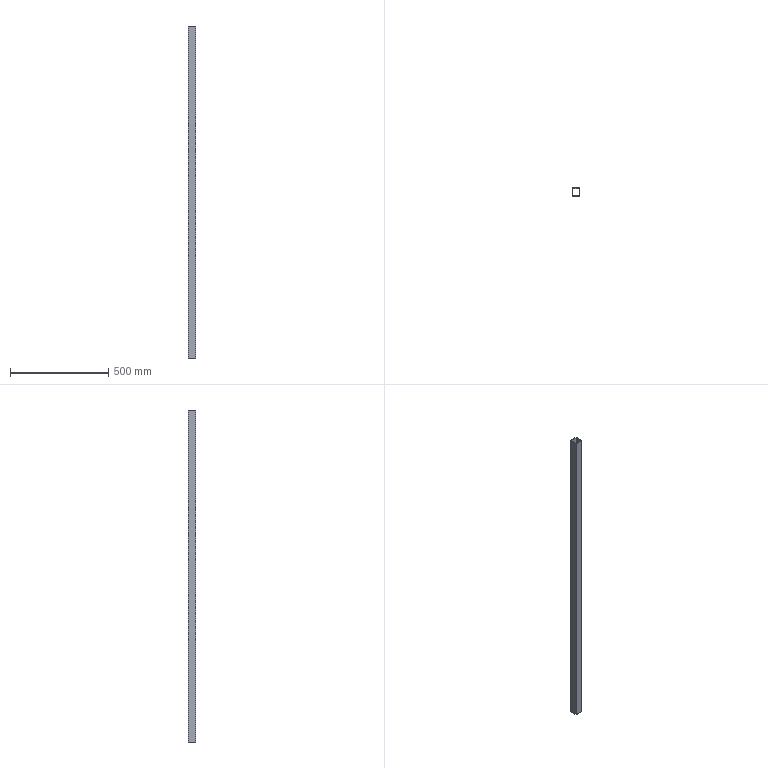Part | STEP file | BCC3 H18_6 | 1 solid | 10 faces | box 40 x 40 x 1690 mm | volume 750360 mm3 | plane 10
STEP:
#1=CARTESIAN_POINT('',(0.,0.,0.));
#2=DIRECTION('',(0.,0.,1.));
#3=DIRECTION('',(1.,0.,0.));
#4=AXIS2_PLACEMENT_3D('',#1,#2,#3);
#5=CARTESIAN_POINT('',(-20.,20.,845.));
#6=VERTEX_POINT('',#5);
#7=CARTESIAN_POINT('',(-20.,-20.,845.));
#8=VERTEX_POINT('',#7);
#9=CARTESIAN_POINT('',(-20.,20.,845.));
#10=DIRECTION('',(0.,-1.,0.));
#11=VECTOR('',#10,1.);
#12=LINE('',#9,#11);
#13=CARTESIAN_POINT('',(0.,0.,845.));
#14=DIRECTION('',(0.,0.,1.));
#15=DIRECTION('',(1.,0.,0.));
#16=AXIS2_PLACEMENT_3D('',#13,#14,#15);
#17=PLANE('',#16);
#18=CARTESIAN_POINT('',(-20.,20.));
#19=DIRECTION('',(0.,-1.));
#20=VECTOR('',#19,1.);
#21=LINE('',#18,#20);
#22=(GEOMETRIC_REPRESENTATION_CONTEXT(2)PARAMETRIC_REPRESENTATION_CONTEXT()REPRESENTATION_CONTEXT('',''));
#23=DEFINITIONAL_REPRESENTATION('',(#21),#22);
#24=PCURVE('',#17,#23);
#25=CARTESIAN_POINT('',(-20.,20.,845.));
#26=DIRECTION('',(1.,0.,0.));
#27=DIRECTION('',(0.,1.,0.));
#28=AXIS2_PLACEMENT_3D('',#25,#26,#27);
#29=PLANE('',#28);
#30=CARTESIAN_POINT('',(0.,0.));
#31=DIRECTION('',(-1.,0.));
#32=VECTOR('',#31,1.);
#33=LINE('',#30,#32);
#34=(GEOMETRIC_REPRESENTATION_CONTEXT(2)PARAMETRIC_REPRESENTATION_CONTEXT()REPRESENTATION_CONTEXT('',''));
#35=DEFINITIONAL_REPRESENTATION('',(#33),#34);
#36=PCURVE('',#29,#35);
#37=SURFACE_CURVE('',#12,(#24,#36),.PCURVE_S1.);
#38=EDGE_CURVE('',#6,#8,#37,.T.);
#39=ORIENTED_EDGE('',*,*,#38,.T.);
#40=CARTESIAN_POINT('',(20.,-20.,845.));
#41=VERTEX_POINT('',#40);
#42=CARTESIAN_POINT('',(-20.,-20.,845.));
#43=DIRECTION('',(1.,0.,0.));
#44=VECTOR('',#43,1.);
#45=LINE('',#42,#44);
#46=CARTESIAN_POINT('',(-20.,-20.));
#47=DIRECTION('',(1.,0.));
#48=VECTOR('',#47,1.);
#49=LINE('',#46,#48);
#50=(GEOMETRIC_REPRESENTATION_CONTEXT(2)PARAMETRIC_REPRESENTATION_CONTEXT()REPRESENTATION_CONTEXT('',''));
#51=DEFINITIONAL_REPRESENTATION('',(#49),#50);
#52=PCURVE('',#17,#51);
#53=CARTESIAN_POINT('',(-20.,-20.,845.));
#54=DIRECTION('',(0.,1.,0.));
#55=DIRECTION('',(0.,0.,1.));
#56=AXIS2_PLACEMENT_3D('',#53,#54,#55);
#57=PLANE('',#56);
#58=CARTESIAN_POINT('',(0.,0.));
#59=DIRECTION('',(0.,1.));
#60=VECTOR('',#59,1.);
#61=LINE('',#58,#60);
#62=(GEOMETRIC_REPRESENTATION_CONTEXT(2)PARAMETRIC_REPRESENTATION_CONTEXT()REPRESENTATION_CONTEXT('',''));
#63=DEFINITIONAL_REPRESENTATION('',(#61),#62);
#64=PCURVE('',#57,#63);
#65=SURFACE_CURVE('',#45,(#52,#64),.PCURVE_S1.);
#66=EDGE_CURVE('',#8,#41,#65,.T.);
#67=ORIENTED_EDGE('',*,*,#66,.T.);
#68=CARTESIAN_POINT('',(20.,20.,845.));
#69=VERTEX_POINT('',#68);
#70=CARTESIAN_POINT('',(20.,20.,845.));
#71=DIRECTION('',(0.,1.,0.));
#72=VECTOR('',#71,1.);
#73=LINE('',#70,#72);
#74=CARTESIAN_POINT('',(20.,20.));
#75=DIRECTION('',(0.,1.));
#76=VECTOR('',#75,1.);
#77=LINE('',#74,#76);
#78=(GEOMETRIC_REPRESENTATION_CONTEXT(2)PARAMETRIC_REPRESENTATION_CONTEXT()REPRESENTATION_CONTEXT('',''));
#79=DEFINITIONAL_REPRESENTATION('',(#77),#78);
#80=PCURVE('',#17,#79);
#81=CARTESIAN_POINT('',(20.,20.,845.));
#82=DIRECTION('',(-1.,0.,0.));
#83=DIRECTION('',(0.,-1.,0.));
#84=AXIS2_PLACEMENT_3D('',#81,#82,#83);
#85=PLANE('',#84);
#86=CARTESIAN_POINT('',(0.,0.));
#87=DIRECTION('',(-1.,0.));
#88=VECTOR('',#87,1.);
#89=LINE('',#86,#88);
#90=(GEOMETRIC_REPRESENTATION_CONTEXT(2)PARAMETRIC_REPRESENTATION_CONTEXT()REPRESENTATION_CONTEXT('',''));
#91=DEFINITIONAL_REPRESENTATION('',(#89),#90);
#92=PCURVE('',#85,#91);
#93=SURFACE_CURVE('',#73,(#80,#92),.PCURVE_S1.);
#94=EDGE_CURVE('',#41,#69,#93,.T.);
#95=ORIENTED_EDGE('',*,*,#94,.T.);
#96=CARTESIAN_POINT('',(-20.,20.,845.));
#97=DIRECTION('',(-1.,0.,0.));
#98=VECTOR('',#97,1.);
#99=LINE('',#96,#98);
#100=CARTESIAN_POINT('',(-20.,20.));
#101=DIRECTION('',(-1.,0.));
#102=VECTOR('',#101,1.);
#103=LINE('',#100,#102);
#104=(GEOMETRIC_REPRESENTATION_CONTEXT(2)PARAMETRIC_REPRESENTATION_CONTEXT()REPRESENTATION_CONTEXT('',''));
#105=DEFINITIONAL_REPRESENTATION('',(#103),#104);
#106=PCURVE('',#17,#105);
#107=CARTESIAN_POINT('',(-20.,20.,845.));
#108=DIRECTION('',(0.,-1.,0.));
#109=DIRECTION('',(0.,0.,-1.));
#110=AXIS2_PLACEMENT_3D('',#107,#108,#109);
#111=PLANE('',#110);
#112=CARTESIAN_POINT('',(0.,0.));
#113=DIRECTION('',(0.,-1.));
#114=VECTOR('',#113,1.);
#115=LINE('',#112,#114);
#116=(GEOMETRIC_REPRESENTATION_CONTEXT(2)PARAMETRIC_REPRESENTATION_CONTEXT()REPRESENTATION_CONTEXT('',''));
#117=DEFINITIONAL_REPRESENTATION('',(#115),#116);
#118=PCURVE('',#111,#117);
#119=SURFACE_CURVE('',#99,(#106,#118),.PCURVE_S1.);
#120=EDGE_CURVE('',#69,#6,#119,.T.);
#121=ORIENTED_EDGE('',*,*,#120,.T.);
#122=EDGE_LOOP('',(#39,#67,#95,#121));
#123=FACE_BOUND('',#122,.T.);
#124=CARTESIAN_POINT('',(-17.,-17.,845.));
#125=VERTEX_POINT('',#124);
#126=CARTESIAN_POINT('',(17.,-17.,845.));
#127=VERTEX_POINT('',#126);
#128=CARTESIAN_POINT('',(-17.,-17.,845.));
#129=DIRECTION('',(1.,0.,0.));
#130=VECTOR('',#129,1.);
#131=LINE('',#128,#130);
#132=CARTESIAN_POINT('',(-17.,-17.));
#133=DIRECTION('',(1.,0.));
#134=VECTOR('',#133,1.);
#135=LINE('',#132,#134);
#136=(GEOMETRIC_REPRESENTATION_CONTEXT(2)PARAMETRIC_REPRESENTATION_CONTEXT()REPRESENTATION_CONTEXT('',''));
#137=DEFINITIONAL_REPRESENTATION('',(#135),#136);
#138=PCURVE('',#17,#137);
#139=CARTESIAN_POINT('',(-17.,-17.,845.));
#140=DIRECTION('',(0.,1.,0.));
#141=DIRECTION('',(-1.,0.,0.));
#142=AXIS2_PLACEMENT_3D('',#139,#140,#141);
#143=PLANE('',#142);
#144=CARTESIAN_POINT('',(0.,0.));
#145=DIRECTION('',(-1.,0.));
#146=VECTOR('',#145,1.);
#147=LINE('',#144,#146);
#148=(GEOMETRIC_REPRESENTATION_CONTEXT(2)PARAMETRIC_REPRESENTATION_CONTEXT()REPRESENTATION_CONTEXT('',''));
#149=DEFINITIONAL_REPRESENTATION('',(#147),#148);
#150=PCURVE('',#143,#149);
#151=SURFACE_CURVE('',#131,(#138,#150),.PCURVE_S1.);
#152=EDGE_CURVE('',#125,#127,#151,.T.);
#153=ORIENTED_EDGE('',*,*,#152,.F.);
#154=CARTESIAN_POINT('',(-17.,17.,845.));
#155=VERTEX_POINT('',#154);
#156=CARTESIAN_POINT('',(-17.,17.,845.));
#157=DIRECTION('',(0.,-1.,0.));
#158=VECTOR('',#157,1.);
#159=LINE('',#156,#158);
#160=CARTESIAN_POINT('',(-17.,17.));
#161=DIRECTION('',(0.,-1.));
#162=VECTOR('',#161,1.);
#163=LINE('',#160,#162);
#164=(GEOMETRIC_REPRESENTATION_CONTEXT(2)PARAMETRIC_REPRESENTATION_CONTEXT()REPRESENTATION_CONTEXT('',''));
#165=DEFINITIONAL_REPRESENTATION('',(#163),#164);
#166=PCURVE('',#17,#165);
#167=CARTESIAN_POINT('',(-17.,17.,845.));
#168=DIRECTION('',(1.,0.,0.));
#169=DIRECTION('',(0.,1.,0.));
#170=AXIS2_PLACEMENT_3D('',#167,#168,#169);
#171=PLANE('',#170);
#172=CARTESIAN_POINT('',(0.,0.));
#173=DIRECTION('',(-1.,0.));
#174=VECTOR('',#173,1.);
#175=LINE('',#172,#174);
#176=(GEOMETRIC_REPRESENTATION_CONTEXT(2)PARAMETRIC_REPRESENTATION_CONTEXT()REPRESENTATION_CONTEXT('',''));
#177=DEFINITIONAL_REPRESENTATION('',(#175),#176);
#178=PCURVE('',#171,#177);
#179=SURFACE_CURVE('',#159,(#166,#178),.PCURVE_S1.);
#180=EDGE_CURVE('',#155,#125,#179,.T.);
#181=ORIENTED_EDGE('',*,*,#180,.F.);
#182=CARTESIAN_POINT('',(17.,17.,845.));
#183=VERTEX_POINT('',#182);
#184=CARTESIAN_POINT('',(-17.,17.,845.));
#185=DIRECTION('',(-1.,0.,0.));
#186=VECTOR('',#185,1.);
#187=LINE('',#184,#186);
#188=CARTESIAN_POINT('',(-17.,17.));
#189=DIRECTION('',(-1.,0.));
#190=VECTOR('',#189,1.);
#191=LINE('',#188,#190);
#192=(GEOMETRIC_REPRESENTATION_CONTEXT(2)PARAMETRIC_REPRESENTATION_CONTEXT()REPRESENTATION_CONTEXT('',''));
#193=DEFINITIONAL_REPRESENTATION('',(#191),#192);
#194=PCURVE('',#17,#193);
#195=CARTESIAN_POINT('',(-17.,17.,845.));
#196=DIRECTION('',(0.,-1.,0.));
#197=DIRECTION('',(0.,0.,-1.));
#198=AXIS2_PLACEMENT_3D('',#195,#196,#197);
#199=PLANE('',#198);
#200=CARTESIAN_POINT('',(0.,0.));
#201=DIRECTION('',(0.,-1.));
#202=VECTOR('',#201,1.);
#203=LINE('',#200,#202);
#204=(GEOMETRIC_REPRESENTATION_CONTEXT(2)PARAMETRIC_REPRESENTATION_CONTEXT()REPRESENTATION_CONTEXT('',''));
#205=DEFINITIONAL_REPRESENTATION('',(#203),#204);
#206=PCURVE('',#199,#205);
#207=SURFACE_CURVE('',#187,(#194,#206),.PCURVE_S1.);
#208=EDGE_CURVE('',#183,#155,#207,.T.);
#209=ORIENTED_EDGE('',*,*,#208,.F.);
#210=CARTESIAN_POINT('',(17.,17.,845.));
#211=DIRECTION('',(0.,1.,0.));
#212=VECTOR('',#211,1.);
#213=LINE('',#210,#212);
#214=CARTESIAN_POINT('',(17.,17.));
#215=DIRECTION('',(0.,1.));
#216=VECTOR('',#215,1.);
#217=LINE('',#214,#216);
#218=(GEOMETRIC_REPRESENTATION_CONTEXT(2)PARAMETRIC_REPRESENTATION_CONTEXT()REPRESENTATION_CONTEXT('',''));
#219=DEFINITIONAL_REPRESENTATION('',(#217),#218);
#220=PCURVE('',#17,#219);
#221=CARTESIAN_POINT('',(17.,17.,845.));
#222=DIRECTION('',(-1.,0.,0.));
#223=DIRECTION('',(0.,-1.,0.));
#224=AXIS2_PLACEMENT_3D('',#221,#222,#223);
#225=PLANE('',#224);
#226=CARTESIAN_POINT('',(0.,0.));
#227=DIRECTION('',(-1.,0.));
#228=VECTOR('',#227,1.);
#229=LINE('',#226,#228);
#230=(GEOMETRIC_REPRESENTATION_CONTEXT(2)PARAMETRIC_REPRESENTATION_CONTEXT()REPRESENTATION_CONTEXT('',''));
#231=DEFINITIONAL_REPRESENTATION('',(#229),#230);
#232=PCURVE('',#225,#231);
#233=SURFACE_CURVE('',#213,(#220,#232),.PCURVE_S1.);
#234=EDGE_CURVE('',#127,#183,#233,.T.);
#235=ORIENTED_EDGE('',*,*,#234,.F.);
#236=EDGE_LOOP('',(#153,#181,#209,#235));
#237=FACE_BOUND('',#236,.T.);
#238=ADVANCED_FACE('',(#123,#237),#17,.T.);
#239=CARTESIAN_POINT('',(-20.,20.,-845.));
#240=VERTEX_POINT('',#239);
#241=CARTESIAN_POINT('',(-20.,-20.,-845.));
#242=VERTEX_POINT('',#241);
#243=CARTESIAN_POINT('',(-20.,20.,-845.));
#244=DIRECTION('',(0.,-1.,0.));
#245=VECTOR('',#244,1.);
#246=LINE('',#243,#245);
#247=CARTESIAN_POINT('',(0.,0.,-845.));
#248=DIRECTION('',(0.,0.,1.));
#249=DIRECTION('',(1.,0.,0.));
#250=AXIS2_PLACEMENT_3D('',#247,#248,#249);
#251=PLANE('',#250);
#252=CARTESIAN_POINT('',(-20.,20.));
#253=DIRECTION('',(0.,-1.));
#254=VECTOR('',#253,1.);
#255=LINE('',#252,#254);
#256=(GEOMETRIC_REPRESENTATION_CONTEXT(2)PARAMETRIC_REPRESENTATION_CONTEXT()REPRESENTATION_CONTEXT('',''));
#257=DEFINITIONAL_REPRESENTATION('',(#255),#256);
#258=PCURVE('',#251,#257);
#259=CARTESIAN_POINT('',(0.,-1690.));
#260=DIRECTION('',(-1.,0.));
#261=VECTOR('',#260,1.);
#262=LINE('',#259,#261);
#263=(GEOMETRIC_REPRESENTATION_CONTEXT(2)PARAMETRIC_REPRESENTATION_CONTEXT()REPRESENTATION_CONTEXT('',''));
#264=DEFINITIONAL_REPRESENTATION('',(#262),#263);
#265=PCURVE('',#29,#264);
#266=SURFACE_CURVE('',#246,(#258,#265),.PCURVE_S1.);
#267=EDGE_CURVE('',#240,#242,#266,.T.);
#268=ORIENTED_EDGE('',*,*,#267,.F.);
#269=CARTESIAN_POINT('',(20.,20.,-845.));
#270=VERTEX_POINT('',#269);
#271=CARTESIAN_POINT('',(-20.,20.,-845.));
#272=DIRECTION('',(-1.,0.,0.));
#273=VECTOR('',#272,1.);
#274=LINE('',#271,#273);
#275=CARTESIAN_POINT('',(-20.,20.));
#276=DIRECTION('',(-1.,0.));
#277=VECTOR('',#276,1.);
#278=LINE('',#275,#277);
#279=(GEOMETRIC_REPRESENTATION_CONTEXT(2)PARAMETRIC_REPRESENTATION_CONTEXT()REPRESENTATION_CONTEXT('',''));
#280=DEFINITIONAL_REPRESENTATION('',(#278),#279);
#281=PCURVE('',#251,#280);
#282=CARTESIAN_POINT('',(1690.,0.));
#283=DIRECTION('',(0.,-1.));
#284=VECTOR('',#283,1.);
#285=LINE('',#282,#284);
#286=(GEOMETRIC_REPRESENTATION_CONTEXT(2)PARAMETRIC_REPRESENTATION_CONTEXT()REPRESENTATION_CONTEXT('',''));
#287=DEFINITIONAL_REPRESENTATION('',(#285),#286);
#288=PCURVE('',#111,#287);
#289=SURFACE_CURVE('',#274,(#281,#288),.PCURVE_S1.);
#290=EDGE_CURVE('',#270,#240,#289,.T.);
#291=ORIENTED_EDGE('',*,*,#290,.F.);
#292=CARTESIAN_POINT('',(20.,-20.,-845.));
#293=VERTEX_POINT('',#292);
#294=CARTESIAN_POINT('',(20.,20.,-845.));
#295=DIRECTION('',(0.,1.,0.));
#296=VECTOR('',#295,1.);
#297=LINE('',#294,#296);
#298=CARTESIAN_POINT('',(20.,20.));
#299=DIRECTION('',(0.,1.));
#300=VECTOR('',#299,1.);
#301=LINE('',#298,#300);
#302=(GEOMETRIC_REPRESENTATION_CONTEXT(2)PARAMETRIC_REPRESENTATION_CONTEXT()REPRESENTATION_CONTEXT('',''));
#303=DEFINITIONAL_REPRESENTATION('',(#301),#302);
#304=PCURVE('',#251,#303);
#305=CARTESIAN_POINT('',(0.,-1690.));
#306=DIRECTION('',(-1.,0.));
#307=VECTOR('',#306,1.);
#308=LINE('',#305,#307);
#309=(GEOMETRIC_REPRESENTATION_CONTEXT(2)PARAMETRIC_REPRESENTATION_CONTEXT()REPRESENTATION_CONTEXT('',''));
#310=DEFINITIONAL_REPRESENTATION('',(#308),#309);
#311=PCURVE('',#85,#310);
#312=SURFACE_CURVE('',#297,(#304,#311),.PCURVE_S1.);
#313=EDGE_CURVE('',#293,#270,#312,.T.);
#314=ORIENTED_EDGE('',*,*,#313,.F.);
#315=CARTESIAN_POINT('',(-20.,-20.,-845.));
#316=DIRECTION('',(1.,0.,0.));
#317=VECTOR('',#316,1.);
#318=LINE('',#315,#317);
#319=CARTESIAN_POINT('',(-20.,-20.));
#320=DIRECTION('',(1.,0.));
#321=VECTOR('',#320,1.);
#322=LINE('',#319,#321);
#323=(GEOMETRIC_REPRESENTATION_CONTEXT(2)PARAMETRIC_REPRESENTATION_CONTEXT()REPRESENTATION_CONTEXT('',''));
#324=DEFINITIONAL_REPRESENTATION('',(#322),#323);
#325=PCURVE('',#251,#324);
#326=CARTESIAN_POINT('',(-1690.,0.));
#327=DIRECTION('',(0.,1.));
#328=VECTOR('',#327,1.);
#329=LINE('',#326,#328);
#330=(GEOMETRIC_REPRESENTATION_CONTEXT(2)PARAMETRIC_REPRESENTATION_CONTEXT()REPRESENTATION_CONTEXT('',''));
#331=DEFINITIONAL_REPRESENTATION('',(#329),#330);
#332=PCURVE('',#57,#331);
#333=SURFACE_CURVE('',#318,(#325,#332),.PCURVE_S1.);
#334=EDGE_CURVE('',#242,#293,#333,.T.);
#335=ORIENTED_EDGE('',*,*,#334,.F.);
#336=EDGE_LOOP('',(#268,#291,#314,#335));
#337=FACE_BOUND('',#336,.T.);
#338=CARTESIAN_POINT('',(-17.,17.,-845.));
#339=VERTEX_POINT('',#338);
#340=CARTESIAN_POINT('',(-17.,-17.,-845.));
#341=VERTEX_POINT('',#340);
#342=CARTESIAN_POINT('',(-17.,17.,-845.));
#343=DIRECTION('',(0.,-1.,0.));
#344=VECTOR('',#343,1.);
#345=LINE('',#342,#344);
#346=CARTESIAN_POINT('',(-17.,17.));
#347=DIRECTION('',(0.,-1.));
#348=VECTOR('',#347,1.);
#349=LINE('',#346,#348);
#350=(GEOMETRIC_REPRESENTATION_CONTEXT(2)PARAMETRIC_REPRESENTATION_CONTEXT()REPRESENTATION_CONTEXT('',''));
#351=DEFINITIONAL_REPRESENTATION('',(#349),#350);
#352=PCURVE('',#251,#351);
#353=CARTESIAN_POINT('',(0.,-1690.));
#354=DIRECTION('',(-1.,0.));
#355=VECTOR('',#354,1.);
#356=LINE('',#353,#355);
#357=(GEOMETRIC_REPRESENTATION_CONTEXT(2)PARAMETRIC_REPRESENTATION_CONTEXT()REPRESENTATION_CONTEXT('',''));
#358=DEFINITIONAL_REPRESENTATION('',(#356),#357);
#359=PCURVE('',#171,#358);
#360=SURFACE_CURVE('',#345,(#352,#359),.PCURVE_S1.);
#361=EDGE_CURVE('',#339,#341,#360,.T.);
#362=ORIENTED_EDGE('',*,*,#361,.T.);
#363=CARTESIAN_POINT('',(17.,-17.,-845.));
#364=VERTEX_POINT('',#363);
#365=CARTESIAN_POINT('',(-17.,-17.,-845.));
#366=DIRECTION('',(1.,0.,0.));
#367=VECTOR('',#366,1.);
#368=LINE('',#365,#367);
#369=CARTESIAN_POINT('',(-17.,-17.));
#370=DIRECTION('',(1.,0.));
#371=VECTOR('',#370,1.);
#372=LINE('',#369,#371);
#373=(GEOMETRIC_REPRESENTATION_CONTEXT(2)PARAMETRIC_REPRESENTATION_CONTEXT()REPRESENTATION_CONTEXT('',''));
#374=DEFINITIONAL_REPRESENTATION('',(#372),#373);
#375=PCURVE('',#251,#374);
#376=CARTESIAN_POINT('',(0.,-1690.));
#377=DIRECTION('',(-1.,0.));
#378=VECTOR('',#377,1.);
#379=LINE('',#376,#378);
#380=(GEOMETRIC_REPRESENTATION_CONTEXT(2)PARAMETRIC_REPRESENTATION_CONTEXT()REPRESENTATION_CONTEXT('',''));
#381=DEFINITIONAL_REPRESENTATION('',(#379),#380);
#382=PCURVE('',#143,#381);
#383=SURFACE_CURVE('',#368,(#375,#382),.PCURVE_S1.);
#384=EDGE_CURVE('',#341,#364,#383,.T.);
#385=ORIENTED_EDGE('',*,*,#384,.T.);
#386=CARTESIAN_POINT('',(17.,17.,-845.));
#387=VERTEX_POINT('',#386);
#388=CARTESIAN_POINT('',(17.,17.,-845.));
#389=DIRECTION('',(0.,1.,0.));
#390=VECTOR('',#389,1.);
#391=LINE('',#388,#390);
#392=CARTESIAN_POINT('',(17.,17.));
#393=DIRECTION('',(0.,1.));
#394=VECTOR('',#393,1.);
#395=LINE('',#392,#394);
#396=(GEOMETRIC_REPRESENTATION_CONTEXT(2)PARAMETRIC_REPRESENTATION_CONTEXT()REPRESENTATION_CONTEXT('',''));
#397=DEFINITIONAL_REPRESENTATION('',(#395),#396);
#398=PCURVE('',#251,#397);
#399=CARTESIAN_POINT('',(0.,-1690.));
#400=DIRECTION('',(-1.,0.));
#401=VECTOR('',#400,1.);
#402=LINE('',#399,#401);
#403=(GEOMETRIC_REPRESENTATION_CONTEXT(2)PARAMETRIC_REPRESENTATION_CONTEXT()REPRESENTATION_CONTEXT('',''));
#404=DEFINITIONAL_REPRESENTATION('',(#402),#403);
#405=PCURVE('',#225,#404);
#406=SURFACE_CURVE('',#391,(#398,#405),.PCURVE_S1.);
#407=EDGE_CURVE('',#364,#387,#406,.T.);
#408=ORIENTED_EDGE('',*,*,#407,.T.);
#409=CARTESIAN_POINT('',(-17.,17.,-845.));
#410=DIRECTION('',(-1.,0.,0.));
#411=VECTOR('',#410,1.);
#412=LINE('',#409,#411);
#413=CARTESIAN_POINT('',(-17.,17.));
#414=DIRECTION('',(-1.,0.));
#415=VECTOR('',#414,1.);
#416=LINE('',#413,#415);
#417=(GEOMETRIC_REPRESENTATION_CONTEXT(2)PARAMETRIC_REPRESENTATION_CONTEXT()REPRESENTATION_CONTEXT('',''));
#418=DEFINITIONAL_REPRESENTATION('',(#416),#417);
#419=PCURVE('',#251,#418);
#420=CARTESIAN_POINT('',(1690.,0.));
#421=DIRECTION('',(0.,-1.));
#422=VECTOR('',#421,1.);
#423=LINE('',#420,#422);
#424=(GEOMETRIC_REPRESENTATION_CONTEXT(2)PARAMETRIC_REPRESENTATION_CONTEXT()REPRESENTATION_CONTEXT('',''));
#425=DEFINITIONAL_REPRESENTATION('',(#423),#424);
#426=PCURVE('',#199,#425);
#427=SURFACE_CURVE('',#412,(#419,#426),.PCURVE_S1.);
#428=EDGE_CURVE('',#387,#339,#427,.T.);
#429=ORIENTED_EDGE('',*,*,#428,.T.);
#430=EDGE_LOOP('',(#362,#385,#408,#429));
#431=FACE_BOUND('',#430,.T.);
#432=ADVANCED_FACE('',(#337,#431),#251,.F.);
#433=ORIENTED_EDGE('',*,*,#267,.T.);
#434=CARTESIAN_POINT('',(-20.,-20.,845.));
#435=DIRECTION('',(0.,0.,-1.));
#436=VECTOR('',#435,1.);
#437=LINE('',#434,#436);
#438=CARTESIAN_POINT('',(-40.,0.));
#439=DIRECTION('',(0.,-1.));
#440=VECTOR('',#439,1.);
#441=LINE('',#438,#440);
#442=(GEOMETRIC_REPRESENTATION_CONTEXT(2)PARAMETRIC_REPRESENTATION_CONTEXT()REPRESENTATION_CONTEXT('',''));
#443=DEFINITIONAL_REPRESENTATION('',(#441),#442);
#444=PCURVE('',#29,#443);
#445=CARTESIAN_POINT('',(0.,0.));
#446=DIRECTION('',(-1.,0.));
#447=VECTOR('',#446,1.);
#448=LINE('',#445,#447);
#449=(GEOMETRIC_REPRESENTATION_CONTEXT(2)PARAMETRIC_REPRESENTATION_CONTEXT()REPRESENTATION_CONTEXT('',''));
#450=DEFINITIONAL_REPRESENTATION('',(#448),#449);
#451=PCURVE('',#57,#450);
#452=SURFACE_CURVE('',#437,(#444,#451),.PCURVE_S1.);
#453=EDGE_CURVE('',#8,#242,#452,.T.);
#454=ORIENTED_EDGE('',*,*,#453,.F.);
#455=ORIENTED_EDGE('',*,*,#38,.F.);
#456=CARTESIAN_POINT('',(-20.,20.,845.));
#457=DIRECTION('',(0.,0.,-1.));
#458=VECTOR('',#457,1.);
#459=LINE('',#456,#458);
#460=CARTESIAN_POINT('',(0.,0.));
#461=DIRECTION('',(0.,-1.));
#462=VECTOR('',#461,1.);
#463=LINE('',#460,#462);
#464=(GEOMETRIC_REPRESENTATION_CONTEXT(2)PARAMETRIC_REPRESENTATION_CONTEXT()REPRESENTATION_CONTEXT('',''));
#465=DEFINITIONAL_REPRESENTATION('',(#463),#464);
#466=PCURVE('',#29,#465);
#467=CARTESIAN_POINT('',(0.,0.));
#468=DIRECTION('',(1.,0.));
#469=VECTOR('',#468,1.);
#470=LINE('',#467,#469);
#471=(GEOMETRIC_REPRESENTATION_CONTEXT(2)PARAMETRIC_REPRESENTATION_CONTEXT()REPRESENTATION_CONTEXT('',''));
#472=DEFINITIONAL_REPRESENTATION('',(#470),#471);
#473=PCURVE('',#111,#472);
#474=SURFACE_CURVE('',#459,(#466,#473),.PCURVE_S1.);
#475=EDGE_CURVE('',#6,#240,#474,.T.);
#476=ORIENTED_EDGE('',*,*,#475,.T.);
#477=EDGE_LOOP('',(#433,#454,#455,#476));
#478=FACE_BOUND('',#477,.T.);
#479=ADVANCED_FACE('',(#478),#29,.F.);
#480=ORIENTED_EDGE('',*,*,#334,.T.);
#481=CARTESIAN_POINT('',(20.,-20.,845.));
#482=DIRECTION('',(0.,0.,-1.));
#483=VECTOR('',#482,1.);
#484=LINE('',#481,#483);
#485=CARTESIAN_POINT('',(0.,40.));
#486=DIRECTION('',(-1.,0.));
#487=VECTOR('',#486,1.);
#488=LINE('',#485,#487);
#489=(GEOMETRIC_REPRESENTATION_CONTEXT(2)PARAMETRIC_REPRESENTATION_CONTEXT()REPRESENTATION_CONTEXT('',''));
#490=DEFINITIONAL_REPRESENTATION('',(#488),#489);
#491=PCURVE('',#57,#490);
#492=CARTESIAN_POINT('',(40.,0.));
#493=DIRECTION('',(0.,-1.));
#494=VECTOR('',#493,1.);
#495=LINE('',#492,#494);
#496=(GEOMETRIC_REPRESENTATION_CONTEXT(2)PARAMETRIC_REPRESENTATION_CONTEXT()REPRESENTATION_CONTEXT('',''));
#497=DEFINITIONAL_REPRESENTATION('',(#495),#496);
#498=PCURVE('',#85,#497);
#499=SURFACE_CURVE('',#484,(#491,#498),.PCURVE_S1.);
#500=EDGE_CURVE('',#41,#293,#499,.T.);
#501=ORIENTED_EDGE('',*,*,#500,.F.);
#502=ORIENTED_EDGE('',*,*,#66,.F.);
#503=ORIENTED_EDGE('',*,*,#453,.T.);
#504=EDGE_LOOP('',(#480,#501,#502,#503));
#505=FACE_BOUND('',#504,.T.);
#506=ADVANCED_FACE('',(#505),#57,.F.);
#507=ORIENTED_EDGE('',*,*,#313,.T.);
#508=CARTESIAN_POINT('',(20.,20.,845.));
#509=DIRECTION('',(0.,0.,-1.));
#510=VECTOR('',#509,1.);
#511=LINE('',#508,#510);
#512=CARTESIAN_POINT('',(0.,0.));
#513=DIRECTION('',(0.,-1.));
#514=VECTOR('',#513,1.);
#515=LINE('',#512,#514);
#516=(GEOMETRIC_REPRESENTATION_CONTEXT(2)PARAMETRIC_REPRESENTATION_CONTEXT()REPRESENTATION_CONTEXT('',''));
#517=DEFINITIONAL_REPRESENTATION('',(#515),#516);
#518=PCURVE('',#85,#517);
#519=CARTESIAN_POINT('',(0.,40.));
#520=DIRECTION('',(1.,0.));
#521=VECTOR('',#520,1.);
#522=LINE('',#519,#521);
#523=(GEOMETRIC_REPRESENTATION_CONTEXT(2)PARAMETRIC_REPRESENTATION_CONTEXT()REPRESENTATION_CONTEXT('',''));
#524=DEFINITIONAL_REPRESENTATION('',(#522),#523);
#525=PCURVE('',#111,#524);
#526=SURFACE_CURVE('',#511,(#518,#525),.PCURVE_S1.);
#527=EDGE_CURVE('',#69,#270,#526,.T.);
#528=ORIENTED_EDGE('',*,*,#527,.F.);
#529=ORIENTED_EDGE('',*,*,#94,.F.);
#530=ORIENTED_EDGE('',*,*,#500,.T.);
#531=EDGE_LOOP('',(#507,#528,#529,#530));
#532=FACE_BOUND('',#531,.T.);
#533=ADVANCED_FACE('',(#532),#85,.F.);
#534=ORIENTED_EDGE('',*,*,#290,.T.);
#535=ORIENTED_EDGE('',*,*,#475,.F.);
#536=ORIENTED_EDGE('',*,*,#120,.F.);
#537=ORIENTED_EDGE('',*,*,#527,.T.);
#538=EDGE_LOOP('',(#534,#535,#536,#537));
#539=FACE_BOUND('',#538,.T.);
#540=ADVANCED_FACE('',(#539),#111,.F.);
#541=ORIENTED_EDGE('',*,*,#361,.F.);
#542=CARTESIAN_POINT('',(-17.,17.,845.));
#543=DIRECTION('',(0.,0.,-1.));
#544=VECTOR('',#543,1.);
#545=LINE('',#542,#544);
#546=CARTESIAN_POINT('',(0.,0.));
#547=DIRECTION('',(0.,-1.));
#548=VECTOR('',#547,1.);
#549=LINE('',#546,#548);
#550=(GEOMETRIC_REPRESENTATION_CONTEXT(2)PARAMETRIC_REPRESENTATION_CONTEXT()REPRESENTATION_CONTEXT('',''));
#551=DEFINITIONAL_REPRESENTATION('',(#549),#550);
#552=PCURVE('',#171,#551);
#553=CARTESIAN_POINT('',(0.,0.));
#554=DIRECTION('',(1.,0.));
#555=VECTOR('',#554,1.);
#556=LINE('',#553,#555);
#557=(GEOMETRIC_REPRESENTATION_CONTEXT(2)PARAMETRIC_REPRESENTATION_CONTEXT()REPRESENTATION_CONTEXT('',''));
#558=DEFINITIONAL_REPRESENTATION('',(#556),#557);
#559=PCURVE('',#199,#558);
#560=SURFACE_CURVE('',#545,(#552,#559),.PCURVE_S1.);
#561=EDGE_CURVE('',#155,#339,#560,.T.);
#562=ORIENTED_EDGE('',*,*,#561,.F.);
#563=ORIENTED_EDGE('',*,*,#180,.T.);
#564=CARTESIAN_POINT('',(-17.,-17.,845.));
#565=DIRECTION('',(0.,0.,-1.));
#566=VECTOR('',#565,1.);
#567=LINE('',#564,#566);
#568=CARTESIAN_POINT('',(-34.,0.));
#569=DIRECTION('',(0.,-1.));
#570=VECTOR('',#569,1.);
#571=LINE('',#568,#570);
#572=(GEOMETRIC_REPRESENTATION_CONTEXT(2)PARAMETRIC_REPRESENTATION_CONTEXT()REPRESENTATION_CONTEXT('',''));
#573=DEFINITIONAL_REPRESENTATION('',(#571),#572);
#574=PCURVE('',#171,#573);
#575=CARTESIAN_POINT('',(0.,0.));
#576=DIRECTION('',(0.,-1.));
#577=VECTOR('',#576,1.);
#578=LINE('',#575,#577);
#579=(GEOMETRIC_REPRESENTATION_CONTEXT(2)PARAMETRIC_REPRESENTATION_CONTEXT()REPRESENTATION_CONTEXT('',''));
#580=DEFINITIONAL_REPRESENTATION('',(#578),#579);
#581=PCURVE('',#143,#580);
#582=SURFACE_CURVE('',#567,(#574,#581),.PCURVE_S1.);
#583=EDGE_CURVE('',#125,#341,#582,.T.);
#584=ORIENTED_EDGE('',*,*,#583,.T.);
#585=EDGE_LOOP('',(#541,#562,#563,#584));
#586=FACE_BOUND('',#585,.T.);
#587=ADVANCED_FACE('',(#586),#171,.T.);
#588=ORIENTED_EDGE('',*,*,#384,.F.);
#589=ORIENTED_EDGE('',*,*,#583,.F.);
#590=ORIENTED_EDGE('',*,*,#152,.T.);
#591=CARTESIAN_POINT('',(17.,-17.,845.));
#592=DIRECTION('',(0.,0.,-1.));
#593=VECTOR('',#592,1.);
#594=LINE('',#591,#593);
#595=CARTESIAN_POINT('',(-34.,0.));
#596=DIRECTION('',(0.,-1.));
#597=VECTOR('',#596,1.);
#598=LINE('',#595,#597);
#599=(GEOMETRIC_REPRESENTATION_CONTEXT(2)PARAMETRIC_REPRESENTATION_CONTEXT()REPRESENTATION_CONTEXT('',''));
#600=DEFINITIONAL_REPRESENTATION('',(#598),#599);
#601=PCURVE('',#143,#600);
#602=CARTESIAN_POINT('',(34.,0.));
#603=DIRECTION('',(0.,-1.));
#604=VECTOR('',#603,1.);
#605=LINE('',#602,#604);
#606=(GEOMETRIC_REPRESENTATION_CONTEXT(2)PARAMETRIC_REPRESENTATION_CONTEXT()REPRESENTATION_CONTEXT('',''));
#607=DEFINITIONAL_REPRESENTATION('',(#605),#606);
#608=PCURVE('',#225,#607);
#609=SURFACE_CURVE('',#594,(#601,#608),.PCURVE_S1.);
#610=EDGE_CURVE('',#127,#364,#609,.T.);
#611=ORIENTED_EDGE('',*,*,#610,.T.);
#612=EDGE_LOOP('',(#588,#589,#590,#611));
#613=FACE_BOUND('',#612,.T.);
#614=ADVANCED_FACE('',(#613),#143,.T.);
#615=ORIENTED_EDGE('',*,*,#407,.F.);
#616=ORIENTED_EDGE('',*,*,#610,.F.);
#617=ORIENTED_EDGE('',*,*,#234,.T.);
#618=CARTESIAN_POINT('',(17.,17.,845.));
#619=DIRECTION('',(0.,0.,-1.));
#620=VECTOR('',#619,1.);
#621=LINE('',#618,#620);
#622=CARTESIAN_POINT('',(0.,0.));
#623=DIRECTION('',(0.,-1.));
#624=VECTOR('',#623,1.);
#625=LINE('',#622,#624);
#626=(GEOMETRIC_REPRESENTATION_CONTEXT(2)PARAMETRIC_REPRESENTATION_CONTEXT()REPRESENTATION_CONTEXT('',''));
#627=DEFINITIONAL_REPRESENTATION('',(#625),#626);
#628=PCURVE('',#225,#627);
#629=CARTESIAN_POINT('',(0.,34.));
#630=DIRECTION('',(1.,0.));
#631=VECTOR('',#630,1.);
#632=LINE('',#629,#631);
#633=(GEOMETRIC_REPRESENTATION_CONTEXT(2)PARAMETRIC_REPRESENTATION_CONTEXT()REPRESENTATION_CONTEXT('',''));
#634=DEFINITIONAL_REPRESENTATION('',(#632),#633);
#635=PCURVE('',#199,#634);
#636=SURFACE_CURVE('',#621,(#628,#635),.PCURVE_S1.);
#637=EDGE_CURVE('',#183,#387,#636,.T.);
#638=ORIENTED_EDGE('',*,*,#637,.T.);
#639=EDGE_LOOP('',(#615,#616,#617,#638));
#640=FACE_BOUND('',#639,.T.);
#641=ADVANCED_FACE('',(#640),#225,.T.);
#642=ORIENTED_EDGE('',*,*,#428,.F.);
#643=ORIENTED_EDGE('',*,*,#637,.F.);
#644=ORIENTED_EDGE('',*,*,#208,.T.);
#645=ORIENTED_EDGE('',*,*,#561,.T.);
#646=EDGE_LOOP('',(#642,#643,#644,#645));
#647=FACE_BOUND('',#646,.T.);
#648=ADVANCED_FACE('',(#647),#199,.T.);
#649=CLOSED_SHELL('',(#238,#432,#479,#506,#533,#540,#587,#614,#641,#648));
#650=MANIFOLD_SOLID_BREP('',#649);
#651=(LENGTH_UNIT()NAMED_UNIT(*)SI_UNIT(.MILLI.,.METRE.));
#652=UNCERTAINTY_MEASURE_WITH_UNIT(LENGTH_MEASURE(0.0000001),#651,'','');
#653=(NAMED_UNIT(*)PLANE_ANGLE_UNIT()SI_UNIT($,.RADIAN.));
#654=(NAMED_UNIT(*)SI_UNIT($,.STERADIAN.)SOLID_ANGLE_UNIT());
#655=(GEOMETRIC_REPRESENTATION_CONTEXT(3)GLOBAL_UNCERTAINTY_ASSIGNED_CONTEXT((#652))GLOBAL_UNIT_ASSIGNED_CONTEXT((#651,#653,#654))REPRESENTATION_CONTEXT('',''));
#656=ADVANCED_BREP_SHAPE_REPRESENTATION('',(#4,#650),#655);